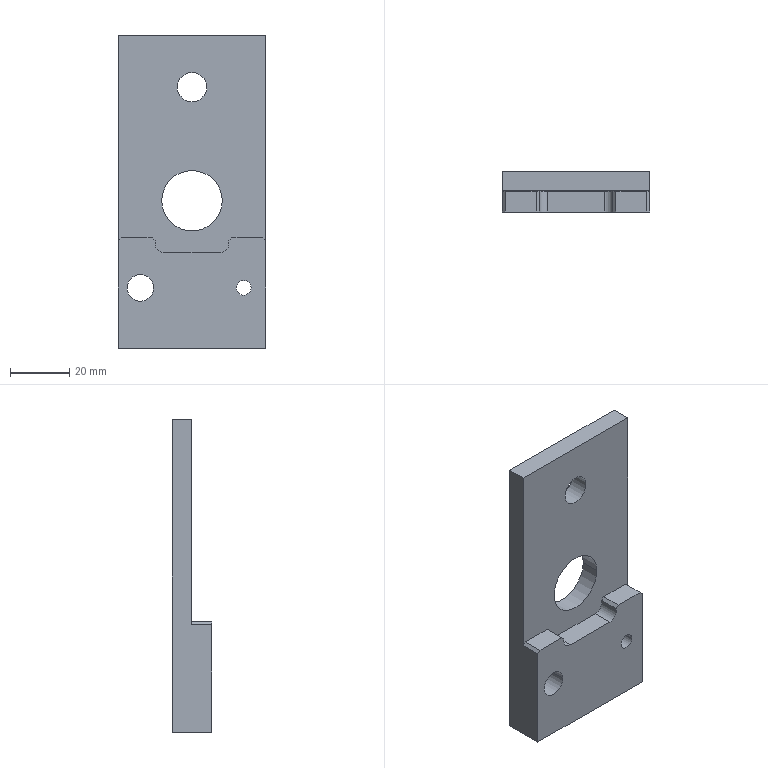Part | NX | features 倒角2 2 | 1 solid | 33 faces | box 50 x 13.5 x 106 mm | volume 42427 mm3 | plane 16 | cylinder 13 | cone 4 | commonest cylinder face diameters 5 x6 6 x2 9 x2 20.5 x2 10 x1
STEP:
#1=CARTESIAN_POINT('',(-22.,342.716,105.381));
#2=VERTEX_POINT('',#1);
#3=CARTESIAN_POINT('',(-13.,342.716,105.381));
#4=VERTEX_POINT('',#3);
#5=CARTESIAN_POINT('',(-17.5,342.716,105.381));
#6=DIRECTION('',(0.,-1.,0.));
#7=DIRECTION('',(1.,0.,0.));
#8=AXIS2_PLACEMENT_3D('',#5,#6,#7);
#9=CIRCLE('',#8,4.5);
#10=EDGE_CURVE('',#2,#4,#9,.T.);
#11=ORIENTED_EDGE('',*,*,#10,.F.);
#12=CARTESIAN_POINT('',(-22.,329.216,105.381));
#13=VERTEX_POINT('',#12);
#14=CARTESIAN_POINT('',(-22.,329.216,105.381));
#15=DIRECTION('',(0.,-1.,0.));
#16=VECTOR('',#15,1000.);
#17=LINE('',#14,#16);
#18=EDGE_CURVE('',#2,#13,#17,.T.);
#19=ORIENTED_EDGE('',*,*,#18,.T.);
#20=CARTESIAN_POINT('',(-13.,329.216,105.381));
#21=VERTEX_POINT('',#20);
#22=CARTESIAN_POINT('',(-17.5,329.216,105.381));
#23=DIRECTION('',(0.,-1.,0.));
#24=DIRECTION('',(1.,0.,0.));
#25=AXIS2_PLACEMENT_3D('',#22,#23,#24);
#26=CIRCLE('',#25,4.5);
#27=EDGE_CURVE('',#13,#21,#26,.T.);
#28=ORIENTED_EDGE('',*,*,#27,.T.);
#29=CARTESIAN_POINT('',(-13.,329.216,105.381));
#30=DIRECTION('',(0.,-1.,0.));
#31=VECTOR('',#30,1000.);
#32=LINE('',#29,#31);
#33=EDGE_CURVE('',#21,#4,#32,.F.);
#34=ORIENTED_EDGE('',*,*,#33,.T.);
#35=EDGE_LOOP('',(#11,#19,#28,#34));
#36=FACE_BOUND('',#35,.T.);
#37=CARTESIAN_POINT('',(-17.5,329.216,105.381));
#38=DIRECTION('',(0.,-1.,0.));
#39=DIRECTION('',(-1.,0.,0.));
#40=AXIS2_PLACEMENT_3D('',#37,#38,#39);
#41=CYLINDRICAL_SURFACE('',#40,4.5);
#42=ADVANCED_FACE('',(#36),#41,.F.);
#43=CARTESIAN_POINT('',(20.,329.216,105.381));
#44=VERTEX_POINT('',#43);
#45=CARTESIAN_POINT('',(15.,329.216,105.381));
#46=VERTEX_POINT('',#45);
#47=CARTESIAN_POINT('',(17.5,329.216,105.381));
#48=DIRECTION('',(0.,1.,0.));
#49=DIRECTION('',(-1.,0.,0.));
#50=AXIS2_PLACEMENT_3D('',#47,#48,#49);
#51=CIRCLE('',#50,2.5);
#52=EDGE_CURVE('',#44,#46,#51,.T.);
#53=ORIENTED_EDGE('',*,*,#52,.F.);
#54=CARTESIAN_POINT('',(20.,342.716,105.381));
#55=VERTEX_POINT('',#54);
#56=CARTESIAN_POINT('',(20.,341.216,105.381));
#57=DIRECTION('',(0.,1.,0.));
#58=VECTOR('',#57,1000.);
#59=LINE('',#56,#58);
#60=EDGE_CURVE('',#55,#44,#59,.F.);
#61=ORIENTED_EDGE('',*,*,#60,.F.);
#62=CARTESIAN_POINT('',(15.,342.716,105.381));
#63=VERTEX_POINT('',#62);
#64=CARTESIAN_POINT('',(17.5,342.716,105.381));
#65=DIRECTION('',(0.,1.,0.));
#66=DIRECTION('',(-1.,0.,0.));
#67=AXIS2_PLACEMENT_3D('',#64,#65,#66);
#68=CIRCLE('',#67,2.5);
#69=EDGE_CURVE('',#55,#63,#68,.T.);
#70=ORIENTED_EDGE('',*,*,#69,.T.);
#71=CARTESIAN_POINT('',(15.,341.216,105.381));
#72=DIRECTION('',(0.,1.,0.));
#73=VECTOR('',#72,1000.);
#74=LINE('',#71,#73);
#75=EDGE_CURVE('',#46,#63,#74,.T.);
#76=ORIENTED_EDGE('',*,*,#75,.F.);
#77=EDGE_LOOP('',(#53,#61,#70,#76));
#78=FACE_BOUND('',#77,.T.);
#79=CARTESIAN_POINT('',(17.5,341.216,105.381));
#80=DIRECTION('',(0.,1.,0.));
#81=DIRECTION('',(1.,0.,0.));
#82=AXIS2_PLACEMENT_3D('',#79,#80,#81);
#83=CYLINDRICAL_SURFACE('',#82,2.5);
#84=ADVANCED_FACE('',(#78),#83,.F.);
#85=CARTESIAN_POINT('',(10.25,342.716,134.881));
#86=VERTEX_POINT('',#85);
#87=CARTESIAN_POINT('',(-10.25,342.716,134.881));
#88=VERTEX_POINT('',#87);
#89=CARTESIAN_POINT('',(-0.000000942,342.716,134.881));
#90=DIRECTION('',(0.,1.,0.));
#91=DIRECTION('',(-1.,0.,0.));
#92=AXIS2_PLACEMENT_3D('',#89,#90,#91);
#93=CIRCLE('',#92,10.25);
#94=EDGE_CURVE('',#86,#88,#93,.T.);
#95=ORIENTED_EDGE('',*,*,#94,.T.);
#96=CARTESIAN_POINT('',(-10.25,336.216,134.881));
#97=VERTEX_POINT('',#96);
#98=CARTESIAN_POINT('',(-10.25,336.216,134.881));
#99=DIRECTION('',(0.,-1.,0.));
#100=VECTOR('',#99,1000.);
#101=LINE('',#98,#100);
#102=EDGE_CURVE('',#88,#97,#101,.T.);
#103=ORIENTED_EDGE('',*,*,#102,.T.);
#104=CARTESIAN_POINT('',(10.25,336.216,134.881));
#105=VERTEX_POINT('',#104);
#106=CARTESIAN_POINT('',(-0.000000942,336.216,134.881));
#107=DIRECTION('',(0.,-1.,0.));
#108=DIRECTION('',(1.,0.,0.));
#109=AXIS2_PLACEMENT_3D('',#106,#107,#108);
#110=CIRCLE('',#109,10.25);
#111=EDGE_CURVE('',#97,#105,#110,.T.);
#112=ORIENTED_EDGE('',*,*,#111,.T.);
#113=CARTESIAN_POINT('',(10.25,336.216,134.881));
#114=DIRECTION('',(0.,-1.,0.));
#115=VECTOR('',#114,1000.);
#116=LINE('',#113,#115);
#117=EDGE_CURVE('',#105,#86,#116,.F.);
#118=ORIENTED_EDGE('',*,*,#117,.T.);
#119=EDGE_LOOP('',(#95,#103,#112,#118));
#120=FACE_BOUND('',#119,.T.);
#121=CARTESIAN_POINT('',(-0.000000942,336.216,134.881));
#122=DIRECTION('',(0.,-1.,0.));
#123=DIRECTION('',(-1.,0.,0.));
#124=AXIS2_PLACEMENT_3D('',#121,#122,#123);
#125=CYLINDRICAL_SURFACE('',#124,10.25);
#126=ADVANCED_FACE('',(#120),#125,.F.);
#127=CARTESIAN_POINT('',(-20.,332.716,97.381));
#128=VERTEX_POINT('',#127);
#129=CARTESIAN_POINT('',(-20.,337.716,97.381));
#130=VERTEX_POINT('',#129);
#131=CARTESIAN_POINT('',(-20.,335.216,97.381));
#132=DIRECTION('',(0.,0.,-1.));
#133=DIRECTION('',(0.,1.,0.));
#134=AXIS2_PLACEMENT_3D('',#131,#132,#133);
#135=CIRCLE('',#134,2.5);
#136=EDGE_CURVE('',#128,#130,#135,.T.);
#137=ORIENTED_EDGE('',*,*,#136,.F.);
#138=CARTESIAN_POINT('',(-20.,332.716,84.866));
#139=VERTEX_POINT('',#138);
#140=CARTESIAN_POINT('',(-20.,332.716,92.381));
#141=DIRECTION('',(0.,0.,-1.));
#142=VECTOR('',#141,1000.);
#143=LINE('',#140,#142);
#144=EDGE_CURVE('',#128,#139,#143,.T.);
#145=ORIENTED_EDGE('',*,*,#144,.T.);
#146=CARTESIAN_POINT('',(-20.,337.716,84.866));
#147=VERTEX_POINT('',#146);
#148=CARTESIAN_POINT('',(-20.,335.216,84.866));
#149=DIRECTION('',(0.000000009,0.,1.));
#150=DIRECTION('',(1.,0.,-0.000000009));
#151=AXIS2_PLACEMENT_3D('',#148,#149,#150);
#152=CIRCLE('',#151,2.5);
#153=EDGE_CURVE('',#139,#147,#152,.F.);
#154=ORIENTED_EDGE('',*,*,#153,.T.);
#155=CARTESIAN_POINT('',(-20.,337.716,92.381));
#156=DIRECTION('',(0.,0.,-1.));
#157=VECTOR('',#156,1000.);
#158=LINE('',#155,#157);
#159=EDGE_CURVE('',#147,#130,#158,.F.);
#160=ORIENTED_EDGE('',*,*,#159,.T.);
#161=EDGE_LOOP('',(#137,#145,#154,#160));
#162=FACE_BOUND('',#161,.T.);
#163=CARTESIAN_POINT('',(-20.,335.216,92.381));
#164=DIRECTION('',(0.,0.,-1.));
#165=DIRECTION('',(0.,-1.,0.));
#166=AXIS2_PLACEMENT_3D('',#163,#164,#165);
#167=CYLINDRICAL_SURFACE('',#166,2.5);
#168=ADVANCED_FACE('',(#162),#167,.F.);
#169=CARTESIAN_POINT('',(-20.,335.216,98.883));
#170=VERTEX_POINT('',#169);
#171=CARTESIAN_POINT('',(-20.,337.716,97.381));
#172=DIRECTION('',(0.,0.8572,-0.515));
#173=VECTOR('',#172,1000.);
#174=LINE('',#171,#173);
#175=EDGE_CURVE('',#130,#170,#174,.F.);
#176=ORIENTED_EDGE('',*,*,#175,.T.);
#177=CARTESIAN_POINT('',(-20.,332.716,97.381));
#178=DIRECTION('',(0.,-0.8572,-0.515));
#179=VECTOR('',#178,1000.);
#180=LINE('',#177,#179);
#181=EDGE_CURVE('',#170,#128,#180,.T.);
#182=ORIENTED_EDGE('',*,*,#181,.T.);
#183=ORIENTED_EDGE('',*,*,#136,.T.);
#184=EDGE_LOOP('',(#176,#182,#183));
#185=FACE_BOUND('',#184,.T.);
#186=CARTESIAN_POINT('',(-20.,335.216,97.381));
#187=DIRECTION('',(0.,0.,-1.));
#188=DIRECTION('',(0.,-1.,0.));
#189=AXIS2_PLACEMENT_3D('',#186,#187,#188);
#190=CONICAL_SURFACE('',#189,2.5,1.03);
#191=ADVANCED_FACE('',(#185),#190,.F.);
#192=CARTESIAN_POINT('',(20.,332.716,97.381));
#193=VERTEX_POINT('',#192);
#194=CARTESIAN_POINT('',(20.,337.716,97.381));
#195=VERTEX_POINT('',#194);
#196=CARTESIAN_POINT('',(20.,335.216,97.381));
#197=DIRECTION('',(0.,0.,-1.));
#198=DIRECTION('',(0.,1.,0.));
#199=AXIS2_PLACEMENT_3D('',#196,#197,#198);
#200=CIRCLE('',#199,2.5);
#201=EDGE_CURVE('',#193,#195,#200,.T.);
#202=ORIENTED_EDGE('',*,*,#201,.F.);
#203=CARTESIAN_POINT('',(20.,332.716,84.866));
#204=VERTEX_POINT('',#203);
#205=CARTESIAN_POINT('',(20.,332.716,92.381));
#206=DIRECTION('',(0.,0.,-1.));
#207=VECTOR('',#206,1000.);
#208=LINE('',#205,#207);
#209=EDGE_CURVE('',#204,#193,#208,.F.);
#210=ORIENTED_EDGE('',*,*,#209,.F.);
#211=CARTESIAN_POINT('',(20.,337.716,84.866));
#212=VERTEX_POINT('',#211);
#213=CARTESIAN_POINT('',(20.,335.216,84.866));
#214=DIRECTION('',(0.000000009,0.,1.));
#215=DIRECTION('',(1.,0.,-0.000000009));
#216=AXIS2_PLACEMENT_3D('',#213,#214,#215);
#217=CIRCLE('',#216,2.5);
#218=EDGE_CURVE('',#204,#212,#217,.F.);
#219=ORIENTED_EDGE('',*,*,#218,.T.);
#220=CARTESIAN_POINT('',(20.,337.716,92.381));
#221=DIRECTION('',(0.,0.,-1.));
#222=VECTOR('',#221,1000.);
#223=LINE('',#220,#222);
#224=EDGE_CURVE('',#195,#212,#223,.T.);
#225=ORIENTED_EDGE('',*,*,#224,.F.);
#226=EDGE_LOOP('',(#202,#210,#219,#225));
#227=FACE_BOUND('',#226,.T.);
#228=CARTESIAN_POINT('',(20.,335.216,92.381));
#229=DIRECTION('',(0.,0.,-1.));
#230=DIRECTION('',(0.,-1.,0.));
#231=AXIS2_PLACEMENT_3D('',#228,#229,#230);
#232=CYLINDRICAL_SURFACE('',#231,2.5);
#233=ADVANCED_FACE('',(#227),#232,.F.);
#234=CARTESIAN_POINT('',(20.,335.216,98.883));
#235=VERTEX_POINT('',#234);
#236=CARTESIAN_POINT('',(20.,337.716,97.381));
#237=DIRECTION('',(0.,0.8572,-0.515));
#238=VECTOR('',#237,1000.);
#239=LINE('',#236,#238);
#240=EDGE_CURVE('',#235,#195,#239,.T.);
#241=ORIENTED_EDGE('',*,*,#240,.F.);
#242=CARTESIAN_POINT('',(20.,332.716,97.381));
#243=DIRECTION('',(0.,-0.8572,-0.515));
#244=VECTOR('',#243,1000.);
#245=LINE('',#242,#244);
#246=EDGE_CURVE('',#193,#235,#245,.F.);
#247=ORIENTED_EDGE('',*,*,#246,.F.);
#248=ORIENTED_EDGE('',*,*,#201,.T.);
#249=EDGE_LOOP('',(#241,#247,#248));
#250=FACE_BOUND('',#249,.T.);
#251=CARTESIAN_POINT('',(20.,335.216,97.381));
#252=DIRECTION('',(0.,0.,-1.));
#253=DIRECTION('',(0.,-1.,0.));
#254=AXIS2_PLACEMENT_3D('',#251,#252,#253);
#255=CONICAL_SURFACE('',#254,2.5,1.03);
#256=ADVANCED_FACE('',(#250),#255,.F.);
#257=CARTESIAN_POINT('',(25.,342.716,190.866));
#258=VERTEX_POINT('',#257);
#259=CARTESIAN_POINT('',(-25.,342.716,190.866));
#260=VERTEX_POINT('',#259);
#261=CARTESIAN_POINT('',(0.000000347,342.716,190.866));
#262=DIRECTION('',(-1.,0.,0.000000019));
#263=VECTOR('',#262,1000.);
#264=LINE('',#261,#263);
#265=EDGE_CURVE('',#258,#260,#264,.T.);
#266=ORIENTED_EDGE('',*,*,#265,.T.);
#267=CARTESIAN_POINT('',(-25.,336.216,190.866));
#268=VERTEX_POINT('',#267);
#269=CARTESIAN_POINT('',(-25.,201.966,190.866));
#270=DIRECTION('',(0.,-1.,0.));
#271=VECTOR('',#270,1000.);
#272=LINE('',#269,#271);
#273=EDGE_CURVE('',#260,#268,#272,.T.);
#274=ORIENTED_EDGE('',*,*,#273,.T.);
#275=CARTESIAN_POINT('',(25.,336.216,190.866));
#276=VERTEX_POINT('',#275);
#277=CARTESIAN_POINT('',(58.,336.216,190.866));
#278=DIRECTION('',(-1.,0.,0.000000019));
#279=VECTOR('',#278,1000.);
#280=LINE('',#277,#279);
#281=EDGE_CURVE('',#276,#268,#280,.T.);
#282=ORIENTED_EDGE('',*,*,#281,.F.);
#283=CARTESIAN_POINT('',(25.,329.216,190.866));
#284=DIRECTION('',(0.,-1.,0.));
#285=VECTOR('',#284,1000.);
#286=LINE('',#283,#285);
#287=EDGE_CURVE('',#258,#276,#286,.T.);
#288=ORIENTED_EDGE('',*,*,#287,.F.);
#289=EDGE_LOOP('',(#266,#274,#282,#288));
#290=FACE_BOUND('',#289,.T.);
#291=CARTESIAN_POINT('',(58.,201.966,190.866));
#292=DIRECTION('',(-0.000000019,0.,-1.));
#293=DIRECTION('',(1.,0.,-0.000000019));
#294=AXIS2_PLACEMENT_3D('',#291,#292,#293);
#295=PLANE('',#294);
#296=ADVANCED_FACE('',(#290),#295,.F.);
#297=CARTESIAN_POINT('',(25.,336.216,121.381));
#298=VERTEX_POINT('',#297);
#299=CARTESIAN_POINT('',(25.,336.216,152.381));
#300=DIRECTION('',(0.,0.,1.));
#301=VECTOR('',#300,1000.);
#302=LINE('',#299,#301);
#303=EDGE_CURVE('',#298,#276,#302,.T.);
#304=ORIENTED_EDGE('',*,*,#303,.F.);
#305=CARTESIAN_POINT('',(25.,329.216,121.381));
#306=VERTEX_POINT('',#305);
#307=CARTESIAN_POINT('',(25.,329.216,121.381));
#308=DIRECTION('',(0.,-1.,0.));
#309=VECTOR('',#308,1000.);
#310=LINE('',#307,#309);
#311=EDGE_CURVE('',#298,#306,#310,.T.);
#312=ORIENTED_EDGE('',*,*,#311,.T.);
#313=CARTESIAN_POINT('',(25.,329.216,84.866));
#314=VERTEX_POINT('',#313);
#315=CARTESIAN_POINT('',(25.,329.216,92.381));
#316=DIRECTION('',(0.,0.,1.));
#317=VECTOR('',#316,1000.);
#318=LINE('',#315,#317);
#319=EDGE_CURVE('',#314,#306,#318,.T.);
#320=ORIENTED_EDGE('',*,*,#319,.F.);
#321=CARTESIAN_POINT('',(25.,342.716,84.866));
#322=VERTEX_POINT('',#321);
#323=CARTESIAN_POINT('',(25.,329.216,84.866));
#324=DIRECTION('',(0.,1.,0.));
#325=VECTOR('',#324,1000.);
#326=LINE('',#323,#325);
#327=EDGE_CURVE('',#314,#322,#326,.T.);
#328=ORIENTED_EDGE('',*,*,#327,.T.);
#329=CARTESIAN_POINT('',(25.,342.716,92.381));
#330=DIRECTION('',(0.,0.,1.));
#331=VECTOR('',#330,1000.);
#332=LINE('',#329,#331);
#333=EDGE_CURVE('',#322,#258,#332,.T.);
#334=ORIENTED_EDGE('',*,*,#333,.T.);
#335=ORIENTED_EDGE('',*,*,#287,.T.);
#336=EDGE_LOOP('',(#304,#312,#320,#328,#334,#335));
#337=FACE_BOUND('',#336,.T.);
#338=CARTESIAN_POINT('',(25.,329.216,92.381));
#339=DIRECTION('',(-1.,0.,0.));
#340=DIRECTION('',(0.,1.,0.));
#341=AXIS2_PLACEMENT_3D('',#338,#339,#340);
#342=PLANE('',#341);
#343=ADVANCED_FACE('',(#337),#342,.F.);
#344=CARTESIAN_POINT('',(-25.,329.216,121.381));
#345=VERTEX_POINT('',#344);
#346=CARTESIAN_POINT('',(-25.,329.216,84.866));
#347=VERTEX_POINT('',#346);
#348=CARTESIAN_POINT('',(-25.,329.216,92.381));
#349=DIRECTION('',(0.,0.,-1.));
#350=VECTOR('',#349,1000.);
#351=LINE('',#348,#350);
#352=EDGE_CURVE('',#345,#347,#351,.T.);
#353=ORIENTED_EDGE('',*,*,#352,.F.);
#354=CARTESIAN_POINT('',(-25.,336.216,121.381));
#355=VERTEX_POINT('',#354);
#356=CARTESIAN_POINT('',(-25.,329.216,121.381));
#357=DIRECTION('',(0.,1.,0.));
#358=VECTOR('',#357,1000.);
#359=LINE('',#356,#358);
#360=EDGE_CURVE('',#345,#355,#359,.T.);
#361=ORIENTED_EDGE('',*,*,#360,.T.);
#362=CARTESIAN_POINT('',(-25.,336.216,152.381));
#363=DIRECTION('',(0.,0.,-1.));
#364=VECTOR('',#363,1000.);
#365=LINE('',#362,#364);
#366=EDGE_CURVE('',#268,#355,#365,.T.);
#367=ORIENTED_EDGE('',*,*,#366,.F.);
#368=ORIENTED_EDGE('',*,*,#273,.F.);
#369=CARTESIAN_POINT('',(-25.,342.716,84.866));
#370=VERTEX_POINT('',#369);
#371=CARTESIAN_POINT('',(-25.,342.716,92.381));
#372=DIRECTION('',(0.,0.,-1.));
#373=VECTOR('',#372,1000.);
#374=LINE('',#371,#373);
#375=EDGE_CURVE('',#260,#370,#374,.T.);
#376=ORIENTED_EDGE('',*,*,#375,.T.);
#377=CARTESIAN_POINT('',(-25.,130.666,84.866));
#378=DIRECTION('',(0.,1.,0.));
#379=VECTOR('',#378,1000.);
#380=LINE('',#377,#379);
#381=EDGE_CURVE('',#347,#370,#380,.T.);
#382=ORIENTED_EDGE('',*,*,#381,.F.);
#383=EDGE_LOOP('',(#353,#361,#367,#368,#376,#382));
#384=FACE_BOUND('',#383,.T.);
#385=CARTESIAN_POINT('',(-25.,329.216,92.381));
#386=DIRECTION('',(1.,0.,0.));
#387=DIRECTION('',(0.,-1.,0.));
#388=AXIS2_PLACEMENT_3D('',#385,#386,#387);
#389=PLANE('',#388);
#390=ADVANCED_FACE('',(#384),#389,.F.);
#391=CARTESIAN_POINT('',(-20.,335.216,84.866));
#392=DIRECTION('',(0.000000009,0.,1.));
#393=DIRECTION('',(1.,0.,-0.000000009));
#394=AXIS2_PLACEMENT_3D('',#391,#392,#393);
#395=CIRCLE('',#394,2.5);
#396=EDGE_CURVE('',#147,#139,#395,.F.);
#397=ORIENTED_EDGE('',*,*,#396,.F.);
#398=ORIENTED_EDGE('',*,*,#153,.F.);
#399=EDGE_LOOP('',(#397,#398));
#400=FACE_BOUND('',#399,.T.);
#401=CARTESIAN_POINT('',(20.,335.216,84.866));
#402=DIRECTION('',(0.000000009,0.,1.));
#403=DIRECTION('',(1.,0.,-0.000000009));
#404=AXIS2_PLACEMENT_3D('',#401,#402,#403);
#405=CIRCLE('',#404,2.5);
#406=EDGE_CURVE('',#212,#204,#405,.F.);
#407=ORIENTED_EDGE('',*,*,#406,.F.);
#408=ORIENTED_EDGE('',*,*,#218,.F.);
#409=EDGE_LOOP('',(#407,#408));
#410=FACE_BOUND('',#409,.T.);
#411=CARTESIAN_POINT('',(-0.000001296,342.716,84.866));
#412=DIRECTION('',(1.,0.,-0.000000009));
#413=VECTOR('',#412,1000.);
#414=LINE('',#411,#413);
#415=EDGE_CURVE('',#370,#322,#414,.T.);
#416=ORIENTED_EDGE('',*,*,#415,.T.);
#417=ORIENTED_EDGE('',*,*,#327,.F.);
#418=CARTESIAN_POINT('',(-0.000001296,329.216,84.866));
#419=DIRECTION('',(1.,0.,-0.000000009));
#420=VECTOR('',#419,1000.);
#421=LINE('',#418,#420);
#422=EDGE_CURVE('',#347,#314,#421,.T.);
#423=ORIENTED_EDGE('',*,*,#422,.F.);
#424=ORIENTED_EDGE('',*,*,#381,.T.);
#425=EDGE_LOOP('',(#416,#417,#423,#424));
#426=FACE_BOUND('',#425,.T.);
#427=CARTESIAN_POINT('',(-25.,130.666,84.866));
#428=DIRECTION('',(0.000000009,0.,1.));
#429=DIRECTION('',(0.,1.,0.));
#430=AXIS2_PLACEMENT_3D('',#427,#428,#429);
#431=PLANE('',#430);
#432=ADVANCED_FACE('',(#400,#410,#426),#431,.F.);
#433=CARTESIAN_POINT('',(-17.5,329.216,105.381));
#434=DIRECTION('',(0.,-1.,0.));
#435=DIRECTION('',(1.,0.,0.));
#436=AXIS2_PLACEMENT_3D('',#433,#434,#435);
#437=CIRCLE('',#436,4.5);
#438=EDGE_CURVE('',#21,#13,#437,.T.);
#439=ORIENTED_EDGE('',*,*,#438,.F.);
#440=ORIENTED_EDGE('',*,*,#27,.F.);
#441=EDGE_LOOP('',(#439,#440));
#442=FACE_BOUND('',#441,.T.);
#443=CARTESIAN_POINT('',(17.5,329.216,105.381));
#444=DIRECTION('',(0.,1.,0.));
#445=DIRECTION('',(-1.,0.,0.));
#446=AXIS2_PLACEMENT_3D('',#443,#444,#445);
#447=CIRCLE('',#446,2.5);
#448=EDGE_CURVE('',#46,#44,#447,.T.);
#449=ORIENTED_EDGE('',*,*,#448,.T.);
#450=ORIENTED_EDGE('',*,*,#52,.T.);
#451=EDGE_LOOP('',(#449,#450));
#452=FACE_BOUND('',#451,.T.);
#453=ORIENTED_EDGE('',*,*,#319,.T.);
#454=CARTESIAN_POINT('',(24.,329.216,122.381));
#455=VERTEX_POINT('',#454);
#456=CARTESIAN_POINT('',(25.,329.216,121.381));
#457=DIRECTION('',(-0.7071,0.,0.7071));
#458=VECTOR('',#457,1000.);
#459=LINE('',#456,#458);
#460=EDGE_CURVE('',#306,#455,#459,.T.);
#461=ORIENTED_EDGE('',*,*,#460,.T.);
#462=CARTESIAN_POINT('',(13.5,329.216,122.381));
#463=VERTEX_POINT('',#462);
#464=CARTESIAN_POINT('',(25.,329.216,122.381));
#465=DIRECTION('',(1.,0.,0.));
#466=VECTOR('',#465,1000.);
#467=LINE('',#464,#466);
#468=EDGE_CURVE('',#463,#455,#467,.T.);
#469=ORIENTED_EDGE('',*,*,#468,.F.);
#470=CARTESIAN_POINT('',(12.5,329.216,121.381));
#471=VERTEX_POINT('',#470);
#472=CARTESIAN_POINT('',(13.5,329.216,122.381));
#473=DIRECTION('',(-0.7071,0.,-0.7071));
#474=VECTOR('',#473,1000.);
#475=LINE('',#472,#474);
#476=EDGE_CURVE('',#463,#471,#475,.T.);
#477=ORIENTED_EDGE('',*,*,#476,.T.);
#478=CARTESIAN_POINT('',(12.5,329.216,120.381));
#479=VERTEX_POINT('',#478);
#480=CARTESIAN_POINT('',(12.5,329.216,122.381));
#481=DIRECTION('',(0.,0.,1.));
#482=VECTOR('',#481,1000.);
#483=LINE('',#480,#482);
#484=EDGE_CURVE('',#479,#471,#483,.T.);
#485=ORIENTED_EDGE('',*,*,#484,.F.);
#486=CARTESIAN_POINT('',(9.5,329.216,117.381));
#487=VERTEX_POINT('',#486);
#488=CARTESIAN_POINT('',(9.5,329.216,120.381));
#489=DIRECTION('',(0.,1.,0.));
#490=DIRECTION('',(-1.,0.,0.));
#491=AXIS2_PLACEMENT_3D('',#488,#489,#490);
#492=CIRCLE('',#491,3.);
#493=EDGE_CURVE('',#479,#487,#492,.T.);
#494=ORIENTED_EDGE('',*,*,#493,.T.);
#495=CARTESIAN_POINT('',(-9.5,329.216,117.381));
#496=VERTEX_POINT('',#495);
#497=CARTESIAN_POINT('',(-12.5,329.216,117.381));
#498=DIRECTION('',(1.,0.,0.));
#499=VECTOR('',#498,1000.);
#500=LINE('',#497,#499);
#501=EDGE_CURVE('',#496,#487,#500,.T.);
#502=ORIENTED_EDGE('',*,*,#501,.F.);
#503=CARTESIAN_POINT('',(-12.5,329.216,120.381));
#504=VERTEX_POINT('',#503);
#505=CARTESIAN_POINT('',(-9.5,329.216,120.381));
#506=DIRECTION('',(0.,1.,0.));
#507=DIRECTION('',(-1.,0.,0.));
#508=AXIS2_PLACEMENT_3D('',#505,#506,#507);
#509=CIRCLE('',#508,3.);
#510=EDGE_CURVE('',#496,#504,#509,.T.);
#511=ORIENTED_EDGE('',*,*,#510,.T.);
#512=CARTESIAN_POINT('',(-12.5,329.216,121.381));
#513=VERTEX_POINT('',#512);
#514=CARTESIAN_POINT('',(-12.5,329.216,122.381));
#515=DIRECTION('',(0.,0.,-1.));
#516=VECTOR('',#515,1000.);
#517=LINE('',#514,#516);
#518=EDGE_CURVE('',#513,#504,#517,.T.);
#519=ORIENTED_EDGE('',*,*,#518,.F.);
#520=CARTESIAN_POINT('',(-13.5,329.216,122.381));
#521=VERTEX_POINT('',#520);
#522=CARTESIAN_POINT('',(-12.5,329.216,121.381));
#523=DIRECTION('',(-0.7071,0.,0.7071));
#524=VECTOR('',#523,1000.);
#525=LINE('',#522,#524);
#526=EDGE_CURVE('',#513,#521,#525,.T.);
#527=ORIENTED_EDGE('',*,*,#526,.T.);
#528=CARTESIAN_POINT('',(-24.,329.216,122.381));
#529=VERTEX_POINT('',#528);
#530=CARTESIAN_POINT('',(-25.,329.216,122.381));
#531=DIRECTION('',(1.,0.,0.));
#532=VECTOR('',#531,1000.);
#533=LINE('',#530,#532);
#534=EDGE_CURVE('',#529,#521,#533,.T.);
#535=ORIENTED_EDGE('',*,*,#534,.F.);
#536=CARTESIAN_POINT('',(-24.,329.216,122.381));
#537=DIRECTION('',(-0.7071,0.,-0.7071));
#538=VECTOR('',#537,1000.);
#539=LINE('',#536,#538);
#540=EDGE_CURVE('',#529,#345,#539,.T.);
#541=ORIENTED_EDGE('',*,*,#540,.T.);
#542=ORIENTED_EDGE('',*,*,#352,.T.);
#543=ORIENTED_EDGE('',*,*,#422,.T.);
#544=EDGE_LOOP('',(#453,#461,#469,#477,#485,#494,#502,#511,#519,#527,#535,#541,#542,#543));
#545=FACE_BOUND('',#544,.T.);
#546=CARTESIAN_POINT('',(-0.000000942,329.216,122.381));
#547=DIRECTION('',(0.,1.,0.));
#548=DIRECTION('',(1.,0.,0.));
#549=AXIS2_PLACEMENT_3D('',#546,#547,#548);
#550=PLANE('',#549);
#551=ADVANCED_FACE('',(#442,#452,#545),#550,.F.);
#552=CARTESIAN_POINT('',(0.000006093,342.716,178.366));
#553=VERTEX_POINT('',#552);
#554=CARTESIAN_POINT('',(0.000006093,342.716,173.366));
#555=DIRECTION('',(0.,1.,0.));
#556=DIRECTION('',(0.,0.,1.));
#557=AXIS2_PLACEMENT_3D('',#554,#555,#556);
#558=CIRCLE('',#557,5.);
#559=EDGE_CURVE('',#553,#553,#558,.T.);
#560=ORIENTED_EDGE('',*,*,#559,.F.);
#561=EDGE_LOOP('',(#560));
#562=FACE_BOUND('',#561,.T.);
#563=CARTESIAN_POINT('',(-17.5,342.716,105.381));
#564=DIRECTION('',(0.,-1.,0.));
#565=DIRECTION('',(1.,0.,0.));
#566=AXIS2_PLACEMENT_3D('',#563,#564,#565);
#567=CIRCLE('',#566,4.5);
#568=EDGE_CURVE('',#4,#2,#567,.T.);
#569=ORIENTED_EDGE('',*,*,#568,.T.);
#570=ORIENTED_EDGE('',*,*,#10,.T.);
#571=EDGE_LOOP('',(#569,#570));
#572=FACE_BOUND('',#571,.T.);
#573=CARTESIAN_POINT('',(17.5,342.716,105.381));
#574=DIRECTION('',(0.,1.,0.));
#575=DIRECTION('',(-1.,0.,0.));
#576=AXIS2_PLACEMENT_3D('',#573,#574,#575);
#577=CIRCLE('',#576,2.5);
#578=EDGE_CURVE('',#63,#55,#577,.T.);
#579=ORIENTED_EDGE('',*,*,#578,.F.);
#580=ORIENTED_EDGE('',*,*,#69,.F.);
#581=EDGE_LOOP('',(#579,#580));
#582=FACE_BOUND('',#581,.T.);
#583=ORIENTED_EDGE('',*,*,#94,.F.);
#584=CARTESIAN_POINT('',(-0.000000942,342.716,134.881));
#585=DIRECTION('',(0.,1.,0.));
#586=DIRECTION('',(-1.,0.,0.));
#587=AXIS2_PLACEMENT_3D('',#584,#585,#586);
#588=CIRCLE('',#587,10.25);
#589=EDGE_CURVE('',#88,#86,#588,.T.);
#590=ORIENTED_EDGE('',*,*,#589,.F.);
#591=EDGE_LOOP('',(#583,#590));
#592=FACE_BOUND('',#591,.T.);
#593=ORIENTED_EDGE('',*,*,#375,.F.);
#594=ORIENTED_EDGE('',*,*,#265,.F.);
#595=ORIENTED_EDGE('',*,*,#333,.F.);
#596=ORIENTED_EDGE('',*,*,#415,.F.);
#597=EDGE_LOOP('',(#593,#594,#595,#596));
#598=FACE_BOUND('',#597,.T.);
#599=CARTESIAN_POINT('',(-0.000000942,342.716,122.381));
#600=DIRECTION('',(0.,1.,0.));
#601=DIRECTION('',(1.,0.,0.));
#602=AXIS2_PLACEMENT_3D('',#599,#600,#601);
#603=PLANE('',#602);
#604=ADVANCED_FACE('',(#562,#572,#582,#592,#598),#603,.T.);
#605=ORIENTED_EDGE('',*,*,#468,.T.);
#606=CARTESIAN_POINT('',(24.,336.216,122.381));
#607=VERTEX_POINT('',#606);
#608=CARTESIAN_POINT('',(24.,336.216,122.381));
#609=DIRECTION('',(0.,1.,0.));
#610=VECTOR('',#609,1000.);
#611=LINE('',#608,#610);
#612=EDGE_CURVE('',#455,#607,#611,.T.);
#613=ORIENTED_EDGE('',*,*,#612,.T.);
#614=CARTESIAN_POINT('',(13.5,336.216,122.381));
#615=VERTEX_POINT('',#614);
#616=CARTESIAN_POINT('',(25.,336.216,122.381));
#617=DIRECTION('',(1.,0.,0.));
#618=VECTOR('',#617,1000.);
#619=LINE('',#616,#618);
#620=EDGE_CURVE('',#615,#607,#619,.T.);
#621=ORIENTED_EDGE('',*,*,#620,.F.);
#622=CARTESIAN_POINT('',(13.5,336.216,122.381));
#623=DIRECTION('',(0.,-1.,0.));
#624=VECTOR('',#623,1000.);
#625=LINE('',#622,#624);
#626=EDGE_CURVE('',#615,#463,#625,.T.);
#627=ORIENTED_EDGE('',*,*,#626,.T.);
#628=EDGE_LOOP('',(#605,#613,#621,#627));
#629=FACE_BOUND('',#628,.T.);
#630=CARTESIAN_POINT('',(25.,336.216,122.381));
#631=DIRECTION('',(0.,0.,-1.));
#632=DIRECTION('',(-1.,0.,0.));
#633=AXIS2_PLACEMENT_3D('',#630,#631,#632);
#634=PLANE('',#633);
#635=ADVANCED_FACE('',(#629),#634,.F.);
#636=ORIENTED_EDGE('',*,*,#484,.T.);
#637=CARTESIAN_POINT('',(12.5,336.216,121.381));
#638=VERTEX_POINT('',#637);
#639=CARTESIAN_POINT('',(12.5,336.216,121.381));
#640=DIRECTION('',(0.,1.,0.));
#641=VECTOR('',#640,1000.);
#642=LINE('',#639,#641);
#643=EDGE_CURVE('',#471,#638,#642,.T.);
#644=ORIENTED_EDGE('',*,*,#643,.T.);
#645=CARTESIAN_POINT('',(12.5,336.216,120.381));
#646=VERTEX_POINT('',#645);
#647=CARTESIAN_POINT('',(12.5,336.216,122.381));
#648=DIRECTION('',(0.,0.,1.));
#649=VECTOR('',#648,1000.);
#650=LINE('',#647,#649);
#651=EDGE_CURVE('',#646,#638,#650,.T.);
#652=ORIENTED_EDGE('',*,*,#651,.F.);
#653=CARTESIAN_POINT('',(12.5,329.216,120.381));
#654=DIRECTION('',(0.,-1.,0.));
#655=VECTOR('',#654,1000.);
#656=LINE('',#653,#655);
#657=EDGE_CURVE('',#646,#479,#656,.T.);
#658=ORIENTED_EDGE('',*,*,#657,.T.);
#659=EDGE_LOOP('',(#636,#644,#652,#658));
#660=FACE_BOUND('',#659,.T.);
#661=CARTESIAN_POINT('',(12.5,336.216,122.381));
#662=DIRECTION('',(1.,0.,0.));
#663=DIRECTION('',(0.,0.,-1.));
#664=AXIS2_PLACEMENT_3D('',#661,#662,#663);
#665=PLANE('',#664);
#666=ADVANCED_FACE('',(#660),#665,.F.);
#667=ORIENTED_EDGE('',*,*,#501,.T.);
#668=CARTESIAN_POINT('',(9.5,336.216,117.381));
#669=VERTEX_POINT('',#668);
#670=CARTESIAN_POINT('',(9.5,336.216,117.381));
#671=DIRECTION('',(0.,1.,0.));
#672=VECTOR('',#671,1000.);
#673=LINE('',#670,#672);
#674=EDGE_CURVE('',#487,#669,#673,.T.);
#675=ORIENTED_EDGE('',*,*,#674,.T.);
#676=CARTESIAN_POINT('',(-9.5,336.216,117.381));
#677=VERTEX_POINT('',#676);
#678=CARTESIAN_POINT('',(-12.5,336.216,117.381));
#679=DIRECTION('',(1.,0.,0.));
#680=VECTOR('',#679,1000.);
#681=LINE('',#678,#680);
#682=EDGE_CURVE('',#677,#669,#681,.T.);
#683=ORIENTED_EDGE('',*,*,#682,.F.);
#684=CARTESIAN_POINT('',(-9.5,329.216,117.381));
#685=DIRECTION('',(0.,-1.,0.));
#686=VECTOR('',#685,1000.);
#687=LINE('',#684,#686);
#688=EDGE_CURVE('',#677,#496,#687,.T.);
#689=ORIENTED_EDGE('',*,*,#688,.T.);
#690=EDGE_LOOP('',(#667,#675,#683,#689));
#691=FACE_BOUND('',#690,.T.);
#692=CARTESIAN_POINT('',(-12.5,336.216,117.381));
#693=DIRECTION('',(0.,0.,-1.));
#694=DIRECTION('',(-1.,0.,0.));
#695=AXIS2_PLACEMENT_3D('',#692,#693,#694);
#696=PLANE('',#695);
#697=ADVANCED_FACE('',(#691),#696,.F.);
#698=CARTESIAN_POINT('',(-12.5,336.216,121.381));
#699=VERTEX_POINT('',#698);
#700=CARTESIAN_POINT('',(-12.5,336.216,120.381));
#701=VERTEX_POINT('',#700);
#702=CARTESIAN_POINT('',(-12.5,336.216,122.381));
#703=DIRECTION('',(0.,0.,-1.));
#704=VECTOR('',#703,1000.);
#705=LINE('',#702,#704);
#706=EDGE_CURVE('',#699,#701,#705,.T.);
#707=ORIENTED_EDGE('',*,*,#706,.F.);
#708=CARTESIAN_POINT('',(-12.5,336.216,121.381));
#709=DIRECTION('',(0.,-1.,0.));
#710=VECTOR('',#709,1000.);
#711=LINE('',#708,#710);
#712=EDGE_CURVE('',#699,#513,#711,.T.);
#713=ORIENTED_EDGE('',*,*,#712,.T.);
#714=ORIENTED_EDGE('',*,*,#518,.T.);
#715=CARTESIAN_POINT('',(-12.5,336.216,120.381));
#716=DIRECTION('',(0.,1.,0.));
#717=VECTOR('',#716,1000.);
#718=LINE('',#715,#717);
#719=EDGE_CURVE('',#504,#701,#718,.T.);
#720=ORIENTED_EDGE('',*,*,#719,.T.);
#721=EDGE_LOOP('',(#707,#713,#714,#720));
#722=FACE_BOUND('',#721,.T.);
#723=CARTESIAN_POINT('',(-12.5,336.216,122.381));
#724=DIRECTION('',(-1.,0.,0.));
#725=DIRECTION('',(0.,0.,1.));
#726=AXIS2_PLACEMENT_3D('',#723,#724,#725);
#727=PLANE('',#726);
#728=ADVANCED_FACE('',(#722),#727,.F.);
#729=ORIENTED_EDGE('',*,*,#534,.T.);
#730=CARTESIAN_POINT('',(-13.5,336.216,122.381));
#731=VERTEX_POINT('',#730);
#732=CARTESIAN_POINT('',(-13.5,336.216,122.381));
#733=DIRECTION('',(0.,1.,0.));
#734=VECTOR('',#733,1000.);
#735=LINE('',#732,#734);
#736=EDGE_CURVE('',#521,#731,#735,.T.);
#737=ORIENTED_EDGE('',*,*,#736,.T.);
#738=CARTESIAN_POINT('',(-24.,336.216,122.381));
#739=VERTEX_POINT('',#738);
#740=CARTESIAN_POINT('',(-25.,336.216,122.381));
#741=DIRECTION('',(1.,0.,0.));
#742=VECTOR('',#741,1000.);
#743=LINE('',#740,#742);
#744=EDGE_CURVE('',#739,#731,#743,.T.);
#745=ORIENTED_EDGE('',*,*,#744,.F.);
#746=CARTESIAN_POINT('',(-24.,336.216,122.381));
#747=DIRECTION('',(0.,-1.,0.));
#748=VECTOR('',#747,1000.);
#749=LINE('',#746,#748);
#750=EDGE_CURVE('',#739,#529,#749,.T.);
#751=ORIENTED_EDGE('',*,*,#750,.T.);
#752=EDGE_LOOP('',(#729,#737,#745,#751));
#753=FACE_BOUND('',#752,.T.);
#754=CARTESIAN_POINT('',(-25.,336.216,122.381));
#755=DIRECTION('',(0.,0.,-1.));
#756=DIRECTION('',(-1.,0.,0.));
#757=AXIS2_PLACEMENT_3D('',#754,#755,#756);
#758=PLANE('',#757);
#759=ADVANCED_FACE('',(#753),#758,.F.);
#760=CARTESIAN_POINT('',(0.000006093,336.216,168.366));
#761=VERTEX_POINT('',#760);
#762=CARTESIAN_POINT('',(0.000006093,336.216,173.366));
#763=DIRECTION('',(0.,-1.,0.));
#764=DIRECTION('',(0.,0.,-1.));
#765=AXIS2_PLACEMENT_3D('',#762,#763,#764);
#766=CIRCLE('',#765,5.);
#767=EDGE_CURVE('',#761,#761,#766,.T.);
#768=ORIENTED_EDGE('',*,*,#767,.F.);
#769=EDGE_LOOP('',(#768));
#770=FACE_BOUND('',#769,.T.);
#771=CARTESIAN_POINT('',(-0.000000942,336.216,134.881));
#772=DIRECTION('',(0.,-1.,0.));
#773=DIRECTION('',(1.,0.,0.));
#774=AXIS2_PLACEMENT_3D('',#771,#772,#773);
#775=CIRCLE('',#774,10.25);
#776=EDGE_CURVE('',#105,#97,#775,.T.);
#777=ORIENTED_EDGE('',*,*,#776,.F.);
#778=ORIENTED_EDGE('',*,*,#111,.F.);
#779=EDGE_LOOP('',(#777,#778));
#780=FACE_BOUND('',#779,.T.);
#781=ORIENTED_EDGE('',*,*,#682,.T.);
#782=CARTESIAN_POINT('',(9.5,336.216,120.381));
#783=DIRECTION('',(0.,-1.,0.));
#784=DIRECTION('',(1.,0.,0.));
#785=AXIS2_PLACEMENT_3D('',#782,#783,#784);
#786=CIRCLE('',#785,3.);
#787=EDGE_CURVE('',#669,#646,#786,.T.);
#788=ORIENTED_EDGE('',*,*,#787,.T.);
#789=ORIENTED_EDGE('',*,*,#651,.T.);
#790=CARTESIAN_POINT('',(13.5,336.216,122.381));
#791=DIRECTION('',(0.7071,0.,0.7071));
#792=VECTOR('',#791,1000.);
#793=LINE('',#790,#792);
#794=EDGE_CURVE('',#638,#615,#793,.T.);
#795=ORIENTED_EDGE('',*,*,#794,.T.);
#796=ORIENTED_EDGE('',*,*,#620,.T.);
#797=CARTESIAN_POINT('',(25.,336.216,121.381));
#798=DIRECTION('',(0.7071,0.,-0.7071));
#799=VECTOR('',#798,1000.);
#800=LINE('',#797,#799);
#801=EDGE_CURVE('',#607,#298,#800,.T.);
#802=ORIENTED_EDGE('',*,*,#801,.T.);
#803=ORIENTED_EDGE('',*,*,#303,.T.);
#804=ORIENTED_EDGE('',*,*,#281,.T.);
#805=ORIENTED_EDGE('',*,*,#366,.T.);
#806=CARTESIAN_POINT('',(-24.,336.216,122.381));
#807=DIRECTION('',(0.7071,0.,0.7071));
#808=VECTOR('',#807,1000.);
#809=LINE('',#806,#808);
#810=EDGE_CURVE('',#355,#739,#809,.T.);
#811=ORIENTED_EDGE('',*,*,#810,.T.);
#812=ORIENTED_EDGE('',*,*,#744,.T.);
#813=CARTESIAN_POINT('',(-12.5,336.216,121.381));
#814=DIRECTION('',(0.7071,0.,-0.7071));
#815=VECTOR('',#814,1000.);
#816=LINE('',#813,#815);
#817=EDGE_CURVE('',#731,#699,#816,.T.);
#818=ORIENTED_EDGE('',*,*,#817,.T.);
#819=ORIENTED_EDGE('',*,*,#706,.T.);
#820=CARTESIAN_POINT('',(-9.5,336.216,120.381));
#821=DIRECTION('',(0.,-1.,0.));
#822=DIRECTION('',(1.,0.,0.));
#823=AXIS2_PLACEMENT_3D('',#820,#821,#822);
#824=CIRCLE('',#823,3.);
#825=EDGE_CURVE('',#701,#677,#824,.T.);
#826=ORIENTED_EDGE('',*,*,#825,.T.);
#827=EDGE_LOOP('',(#781,#788,#789,#795,#796,#802,#803,#804,#805,#811,#812,#818,#819,#826));
#828=FACE_BOUND('',#827,.T.);
#829=CARTESIAN_POINT('',(-0.000000942,336.216,122.381));
#830=DIRECTION('',(0.,-1.,0.));
#831=DIRECTION('',(-1.,0.,0.));
#832=AXIS2_PLACEMENT_3D('',#829,#830,#831);
#833=PLANE('',#832);
#834=ADVANCED_FACE('',(#770,#780,#828),#833,.T.);
#835=ORIENTED_EDGE('',*,*,#246,.T.);
#836=ORIENTED_EDGE('',*,*,#240,.T.);
#837=CARTESIAN_POINT('',(20.,335.216,97.381));
#838=DIRECTION('',(0.,0.,-1.));
#839=DIRECTION('',(0.,1.,0.));
#840=AXIS2_PLACEMENT_3D('',#837,#838,#839);
#841=CIRCLE('',#840,2.5);
#842=EDGE_CURVE('',#195,#193,#841,.T.);
#843=ORIENTED_EDGE('',*,*,#842,.T.);
#844=EDGE_LOOP('',(#835,#836,#843));
#845=FACE_BOUND('',#844,.T.);
#846=CARTESIAN_POINT('',(20.,335.216,97.381));
#847=DIRECTION('',(0.,0.,-1.));
#848=DIRECTION('',(0.,-1.,0.));
#849=AXIS2_PLACEMENT_3D('',#846,#847,#848);
#850=CONICAL_SURFACE('',#849,2.5,1.03);
#851=ADVANCED_FACE('',(#845),#850,.F.);
#852=ORIENTED_EDGE('',*,*,#209,.T.);
#853=ORIENTED_EDGE('',*,*,#842,.F.);
#854=ORIENTED_EDGE('',*,*,#224,.T.);
#855=ORIENTED_EDGE('',*,*,#406,.T.);
#856=EDGE_LOOP('',(#852,#853,#854,#855));
#857=FACE_BOUND('',#856,.T.);
#858=CARTESIAN_POINT('',(20.,335.216,92.381));
#859=DIRECTION('',(0.,0.,-1.));
#860=DIRECTION('',(0.,-1.,0.));
#861=AXIS2_PLACEMENT_3D('',#858,#859,#860);
#862=CYLINDRICAL_SURFACE('',#861,2.5);
#863=ADVANCED_FACE('',(#857),#862,.F.);
#864=ORIENTED_EDGE('',*,*,#181,.F.);
#865=ORIENTED_EDGE('',*,*,#175,.F.);
#866=CARTESIAN_POINT('',(-20.,335.216,97.381));
#867=DIRECTION('',(0.,0.,-1.));
#868=DIRECTION('',(0.,1.,0.));
#869=AXIS2_PLACEMENT_3D('',#866,#867,#868);
#870=CIRCLE('',#869,2.5);
#871=EDGE_CURVE('',#130,#128,#870,.T.);
#872=ORIENTED_EDGE('',*,*,#871,.T.);
#873=EDGE_LOOP('',(#864,#865,#872));
#874=FACE_BOUND('',#873,.T.);
#875=CARTESIAN_POINT('',(-20.,335.216,97.381));
#876=DIRECTION('',(0.,0.,-1.));
#877=DIRECTION('',(0.,-1.,0.));
#878=AXIS2_PLACEMENT_3D('',#875,#876,#877);
#879=CONICAL_SURFACE('',#878,2.5,1.03);
#880=ADVANCED_FACE('',(#874),#879,.F.);
#881=ORIENTED_EDGE('',*,*,#144,.F.);
#882=ORIENTED_EDGE('',*,*,#871,.F.);
#883=ORIENTED_EDGE('',*,*,#159,.F.);
#884=ORIENTED_EDGE('',*,*,#396,.T.);
#885=EDGE_LOOP('',(#881,#882,#883,#884));
#886=FACE_BOUND('',#885,.T.);
#887=CARTESIAN_POINT('',(-20.,335.216,92.381));
#888=DIRECTION('',(0.,0.,-1.));
#889=DIRECTION('',(0.,-1.,0.));
#890=AXIS2_PLACEMENT_3D('',#887,#888,#889);
#891=CYLINDRICAL_SURFACE('',#890,2.5);
#892=ADVANCED_FACE('',(#886),#891,.F.);
#893=ORIENTED_EDGE('',*,*,#102,.F.);
#894=ORIENTED_EDGE('',*,*,#589,.T.);
#895=ORIENTED_EDGE('',*,*,#117,.F.);
#896=ORIENTED_EDGE('',*,*,#776,.T.);
#897=EDGE_LOOP('',(#893,#894,#895,#896));
#898=FACE_BOUND('',#897,.T.);
#899=CARTESIAN_POINT('',(-0.000000942,336.216,134.881));
#900=DIRECTION('',(0.,-1.,0.));
#901=DIRECTION('',(-1.,0.,0.));
#902=AXIS2_PLACEMENT_3D('',#899,#900,#901);
#903=CYLINDRICAL_SURFACE('',#902,10.25);
#904=ADVANCED_FACE('',(#898),#903,.F.);
#905=ORIENTED_EDGE('',*,*,#60,.T.);
#906=ORIENTED_EDGE('',*,*,#448,.F.);
#907=ORIENTED_EDGE('',*,*,#75,.T.);
#908=ORIENTED_EDGE('',*,*,#578,.T.);
#909=EDGE_LOOP('',(#905,#906,#907,#908));
#910=FACE_BOUND('',#909,.T.);
#911=CARTESIAN_POINT('',(17.5,341.216,105.381));
#912=DIRECTION('',(0.,1.,0.));
#913=DIRECTION('',(1.,0.,0.));
#914=AXIS2_PLACEMENT_3D('',#911,#912,#913);
#915=CYLINDRICAL_SURFACE('',#914,2.5);
#916=ADVANCED_FACE('',(#910),#915,.F.);
#917=ORIENTED_EDGE('',*,*,#18,.F.);
#918=ORIENTED_EDGE('',*,*,#568,.F.);
#919=ORIENTED_EDGE('',*,*,#33,.F.);
#920=ORIENTED_EDGE('',*,*,#438,.T.);
#921=EDGE_LOOP('',(#917,#918,#919,#920));
#922=FACE_BOUND('',#921,.T.);
#923=CARTESIAN_POINT('',(-17.5,329.216,105.381));
#924=DIRECTION('',(0.,-1.,0.));
#925=DIRECTION('',(-1.,0.,0.));
#926=AXIS2_PLACEMENT_3D('',#923,#924,#925);
#927=CYLINDRICAL_SURFACE('',#926,4.5);
#928=ADVANCED_FACE('',(#922),#927,.F.);
#929=ORIENTED_EDGE('',*,*,#787,.F.);
#930=ORIENTED_EDGE('',*,*,#674,.F.);
#931=ORIENTED_EDGE('',*,*,#493,.F.);
#932=ORIENTED_EDGE('',*,*,#657,.F.);
#933=EDGE_LOOP('',(#929,#930,#931,#932));
#934=FACE_BOUND('',#933,.T.);
#935=CARTESIAN_POINT('',(9.5,336.216,120.381));
#936=DIRECTION('',(0.,1.,0.));
#937=DIRECTION('',(1.,0.,0.));
#938=AXIS2_PLACEMENT_3D('',#935,#936,#937);
#939=CYLINDRICAL_SURFACE('',#938,3.);
#940=ADVANCED_FACE('',(#934),#939,.F.);
#941=ORIENTED_EDGE('',*,*,#825,.F.);
#942=ORIENTED_EDGE('',*,*,#719,.F.);
#943=ORIENTED_EDGE('',*,*,#510,.F.);
#944=ORIENTED_EDGE('',*,*,#688,.F.);
#945=EDGE_LOOP('',(#941,#942,#943,#944));
#946=FACE_BOUND('',#945,.T.);
#947=CARTESIAN_POINT('',(-9.5,336.216,120.381));
#948=DIRECTION('',(0.,1.,0.));
#949=DIRECTION('',(1.,0.,0.));
#950=AXIS2_PLACEMENT_3D('',#947,#948,#949);
#951=CYLINDRICAL_SURFACE('',#950,3.);
#952=ADVANCED_FACE('',(#946),#951,.F.);
#953=ORIENTED_EDGE('',*,*,#801,.F.);
#954=ORIENTED_EDGE('',*,*,#612,.F.);
#955=ORIENTED_EDGE('',*,*,#460,.F.);
#956=ORIENTED_EDGE('',*,*,#311,.F.);
#957=EDGE_LOOP('',(#953,#954,#955,#956));
#958=FACE_BOUND('',#957,.T.);
#959=CARTESIAN_POINT('',(25.,329.216,121.381));
#960=DIRECTION('',(-0.7071,0.,-0.7071));
#961=DIRECTION('',(0.,1.,0.));
#962=AXIS2_PLACEMENT_3D('',#959,#960,#961);
#963=PLANE('',#962);
#964=ADVANCED_FACE('',(#958),#963,.F.);
#965=ORIENTED_EDGE('',*,*,#794,.F.);
#966=ORIENTED_EDGE('',*,*,#643,.F.);
#967=ORIENTED_EDGE('',*,*,#476,.F.);
#968=ORIENTED_EDGE('',*,*,#626,.F.);
#969=EDGE_LOOP('',(#965,#966,#967,#968));
#970=FACE_BOUND('',#969,.T.);
#971=CARTESIAN_POINT('',(13.5,336.216,122.381));
#972=DIRECTION('',(0.7071,0.,-0.7071));
#973=DIRECTION('',(0.,1.,0.));
#974=AXIS2_PLACEMENT_3D('',#971,#972,#973);
#975=PLANE('',#974);
#976=ADVANCED_FACE('',(#970),#975,.F.);
#977=ORIENTED_EDGE('',*,*,#817,.F.);
#978=ORIENTED_EDGE('',*,*,#736,.F.);
#979=ORIENTED_EDGE('',*,*,#526,.F.);
#980=ORIENTED_EDGE('',*,*,#712,.F.);
#981=EDGE_LOOP('',(#977,#978,#979,#980));
#982=FACE_BOUND('',#981,.T.);
#983=CARTESIAN_POINT('',(-12.5,336.216,121.381));
#984=DIRECTION('',(-0.7071,0.,-0.7071));
#985=DIRECTION('',(0.,1.,0.));
#986=AXIS2_PLACEMENT_3D('',#983,#984,#985);
#987=PLANE('',#986);
#988=ADVANCED_FACE('',(#982),#987,.F.);
#989=ORIENTED_EDGE('',*,*,#810,.F.);
#990=ORIENTED_EDGE('',*,*,#360,.F.);
#991=ORIENTED_EDGE('',*,*,#540,.F.);
#992=ORIENTED_EDGE('',*,*,#750,.F.);
#993=EDGE_LOOP('',(#989,#990,#991,#992));
#994=FACE_BOUND('',#993,.T.);
#995=CARTESIAN_POINT('',(-24.,336.216,122.381));
#996=DIRECTION('',(0.7071,0.,-0.7071));
#997=DIRECTION('',(0.,1.,0.));
#998=AXIS2_PLACEMENT_3D('',#995,#996,#997);
#999=PLANE('',#998);
#1000=ADVANCED_FACE('',(#994),#999,.F.);
#1001=ORIENTED_EDGE('',*,*,#559,.T.);
#1002=EDGE_LOOP('',(#1001));
#1003=FACE_BOUND('',#1002,.T.);
#1004=ORIENTED_EDGE('',*,*,#767,.T.);
#1005=EDGE_LOOP('',(#1004));
#1006=FACE_BOUND('',#1005,.T.);
#1007=CARTESIAN_POINT('',(0.000006093,412.332,173.366));
#1008=DIRECTION('',(0.,1.,0.));
#1009=DIRECTION('',(0.8321,0.,-0.5546));
#1010=AXIS2_PLACEMENT_3D('',#1007,#1008,#1009);
#1011=CYLINDRICAL_SURFACE('',#1010,5.);
#1012=ADVANCED_FACE('',(#1003,#1006),#1011,.F.);
#1013=CLOSED_SHELL('',(#42,#84,#126,#168,#191,#233,#256,#296,#343,#390,#432,#551,#604,#635,#666,#697,#728,#759,#834,#851,#863,#880,#892,#904,#916,#928,#940,#952,#964,#976,#988,#1000,#1012));
#1014=MANIFOLD_SOLID_BREP('',#1013);
#1015=(LENGTH_UNIT()NAMED_UNIT(*)SI_UNIT(.MILLI.,.METRE.));
#1016=UNCERTAINTY_MEASURE_WITH_UNIT(LENGTH_MEASURE(0.00001),#1015,'','');
#1017=(NAMED_UNIT(*)PLANE_ANGLE_UNIT()SI_UNIT($,.RADIAN.));
#1018=(NAMED_UNIT(*)SI_UNIT($,.STERADIAN.)SOLID_ANGLE_UNIT());
#1019=(GEOMETRIC_REPRESENTATION_CONTEXT(3)GLOBAL_UNCERTAINTY_ASSIGNED_CONTEXT((#1016))GLOBAL_UNIT_ASSIGNED_CONTEXT((#1015,#1017,#1018))REPRESENTATION_CONTEXT('',''));
#1020=ADVANCED_BREP_SHAPE_REPRESENTATION('',(#1014),#1019);